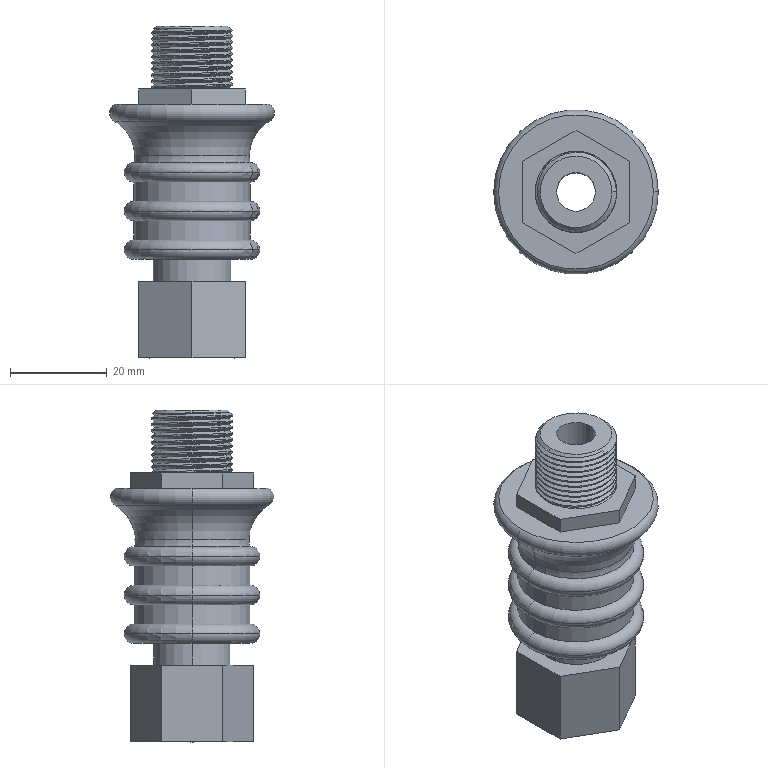Part | NX | 1 solid | 90 faces | box 34 x 34 x 68.54 mm | volume 24989 mm3 | cylinder 32 | plane 28 | torus 18 | cone 6 | spline 6 | commonest cylinder face diameters 16.8 x22 24 x4 8 x2 14 x2 16 x2